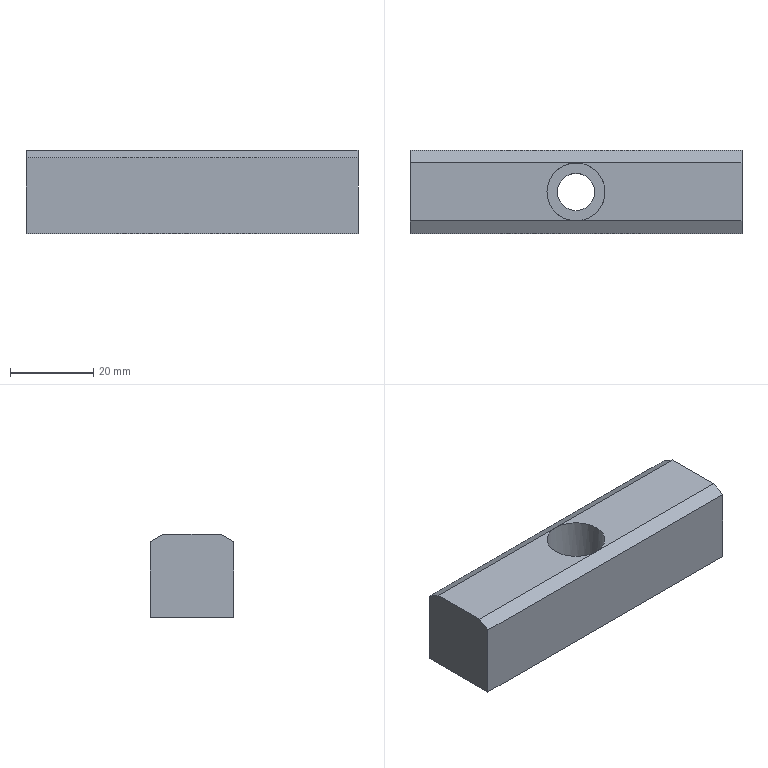Part | NX | features solid 2 | 1 solid | 12 faces | box 80 x 20 x 20 mm | volume 29409 mm3 | plane 10 | cylinder 2 | commonest cylinder face diameters 9 x1 14 x1
STEP:
#1=CARTESIAN_POINT('',(40.,347.,-95.));
#2=VERTEX_POINT('',#1);
#3=CARTESIAN_POINT('',(40.,333.,-95.));
#4=VERTEX_POINT('',#3);
#5=CARTESIAN_POINT('',(40.,350.,-95.));
#6=DIRECTION('',(0.,1.,0.));
#7=VECTOR('',#6,1000.);
#8=LINE('',#5,#7);
#9=EDGE_CURVE('',#2,#4,#8,.F.);
#10=ORIENTED_EDGE('',*,*,#9,.F.);
#11=CARTESIAN_POINT('',(0.,347.,-95.));
#12=VERTEX_POINT('',#11);
#13=CARTESIAN_POINT('',(40.,347.,-95.));
#14=DIRECTION('',(-1.,0.,0.));
#15=VECTOR('',#14,1000.);
#16=LINE('',#13,#15);
#17=EDGE_CURVE('',#2,#12,#16,.T.);
#18=ORIENTED_EDGE('',*,*,#17,.T.);
#19=CARTESIAN_POINT('',(0.,333.,-95.));
#20=VERTEX_POINT('',#19);
#21=CARTESIAN_POINT('',(0.,340.,-95.));
#22=DIRECTION('',(0.,0.,-1.));
#23=DIRECTION('',(-1.,0.,0.));
#24=AXIS2_PLACEMENT_3D('',#21,#22,#23);
#25=CIRCLE('',#24,7.);
#26=EDGE_CURVE('',#12,#20,#25,.T.);
#27=ORIENTED_EDGE('',*,*,#26,.T.);
#28=CARTESIAN_POINT('',(40.,333.,-95.));
#29=DIRECTION('',(1.,0.,0.));
#30=VECTOR('',#29,1000.);
#31=LINE('',#28,#30);
#32=EDGE_CURVE('',#20,#4,#31,.T.);
#33=ORIENTED_EDGE('',*,*,#32,.T.);
#34=EDGE_LOOP('',(#10,#18,#27,#33));
#35=FACE_BOUND('',#34,.T.);
#36=CARTESIAN_POINT('',(40.,350.,-95.));
#37=DIRECTION('',(0.,0.,1.));
#38=DIRECTION('',(1.,0.,0.));
#39=AXIS2_PLACEMENT_3D('',#36,#37,#38);
#40=PLANE('',#39);
#41=ADVANCED_FACE('',(#35),#40,.T.);
#42=CARTESIAN_POINT('',(-40.,350.,-115.));
#43=VERTEX_POINT('',#42);
#44=CARTESIAN_POINT('',(-40.,350.,-96.732));
#45=VERTEX_POINT('',#44);
#46=CARTESIAN_POINT('',(-40.,350.,-115.));
#47=DIRECTION('',(0.,0.,1.));
#48=VECTOR('',#47,1000.);
#49=LINE('',#46,#48);
#50=EDGE_CURVE('',#43,#45,#49,.T.);
#51=ORIENTED_EDGE('',*,*,#50,.T.);
#52=CARTESIAN_POINT('',(40.,350.,-96.732));
#53=VERTEX_POINT('',#52);
#54=CARTESIAN_POINT('',(40.,350.,-96.732));
#55=DIRECTION('',(1.,0.,0.));
#56=VECTOR('',#55,1000.);
#57=LINE('',#54,#56);
#58=EDGE_CURVE('',#45,#53,#57,.T.);
#59=ORIENTED_EDGE('',*,*,#58,.T.);
#60=CARTESIAN_POINT('',(40.,350.,-115.));
#61=VERTEX_POINT('',#60);
#62=CARTESIAN_POINT('',(40.,350.,-115.));
#63=DIRECTION('',(0.,0.,1.));
#64=VECTOR('',#63,1000.);
#65=LINE('',#62,#64);
#66=EDGE_CURVE('',#61,#53,#65,.T.);
#67=ORIENTED_EDGE('',*,*,#66,.F.);
#68=CARTESIAN_POINT('',(40.,350.,-115.));
#69=DIRECTION('',(-1.,0.,0.));
#70=VECTOR('',#69,1000.);
#71=LINE('',#68,#70);
#72=EDGE_CURVE('',#61,#43,#71,.T.);
#73=ORIENTED_EDGE('',*,*,#72,.T.);
#74=EDGE_LOOP('',(#51,#59,#67,#73));
#75=FACE_BOUND('',#74,.T.);
#76=CARTESIAN_POINT('',(40.,350.,-115.));
#77=DIRECTION('',(0.,1.,0.));
#78=DIRECTION('',(-1.,0.,0.));
#79=AXIS2_PLACEMENT_3D('',#76,#77,#78);
#80=PLANE('',#79);
#81=ADVANCED_FACE('',(#75),#80,.T.);
#82=CARTESIAN_POINT('',(-40.,347.,-95.));
#83=VERTEX_POINT('',#82);
#84=CARTESIAN_POINT('',(-40.,333.,-95.));
#85=VERTEX_POINT('',#84);
#86=CARTESIAN_POINT('',(-40.,350.,-95.));
#87=DIRECTION('',(0.,1.,0.));
#88=VECTOR('',#87,1000.);
#89=LINE('',#86,#88);
#90=EDGE_CURVE('',#83,#85,#89,.F.);
#91=ORIENTED_EDGE('',*,*,#90,.F.);
#92=CARTESIAN_POINT('',(-40.,357.91,-101.299));
#93=DIRECTION('',(0.,-0.866,0.5));
#94=VECTOR('',#93,1000.);
#95=LINE('',#92,#94);
#96=EDGE_CURVE('',#83,#45,#95,.F.);
#97=ORIENTED_EDGE('',*,*,#96,.T.);
#98=ORIENTED_EDGE('',*,*,#50,.F.);
#99=CARTESIAN_POINT('',(-40.,330.,-115.));
#100=VERTEX_POINT('',#99);
#101=CARTESIAN_POINT('',(-40.,350.,-115.));
#102=DIRECTION('',(0.,-1.,0.));
#103=VECTOR('',#102,1000.);
#104=LINE('',#101,#103);
#105=EDGE_CURVE('',#43,#100,#104,.T.);
#106=ORIENTED_EDGE('',*,*,#105,.T.);
#107=CARTESIAN_POINT('',(-40.,330.,-96.732));
#108=VERTEX_POINT('',#107);
#109=CARTESIAN_POINT('',(-40.,330.,-115.));
#110=DIRECTION('',(0.,0.,1.));
#111=VECTOR('',#110,1000.);
#112=LINE('',#109,#111);
#113=EDGE_CURVE('',#100,#108,#112,.T.);
#114=ORIENTED_EDGE('',*,*,#113,.T.);
#115=CARTESIAN_POINT('',(-40.,337.09,-92.639));
#116=DIRECTION('',(0.,0.866,0.5));
#117=VECTOR('',#116,1000.);
#118=LINE('',#115,#117);
#119=EDGE_CURVE('',#108,#85,#118,.T.);
#120=ORIENTED_EDGE('',*,*,#119,.T.);
#121=EDGE_LOOP('',(#91,#97,#98,#106,#114,#120));
#122=FACE_BOUND('',#121,.T.);
#123=CARTESIAN_POINT('',(-40.,350.,-115.));
#124=DIRECTION('',(-1.,0.,0.));
#125=DIRECTION('',(0.,-1.,0.));
#126=AXIS2_PLACEMENT_3D('',#123,#124,#125);
#127=PLANE('',#126);
#128=ADVANCED_FACE('',(#122),#127,.T.);
#129=CARTESIAN_POINT('',(40.,330.,-115.));
#130=VERTEX_POINT('',#129);
#131=CARTESIAN_POINT('',(40.,330.,-96.732));
#132=VERTEX_POINT('',#131);
#133=CARTESIAN_POINT('',(40.,330.,-115.));
#134=DIRECTION('',(0.,0.,1.));
#135=VECTOR('',#134,1000.);
#136=LINE('',#133,#135);
#137=EDGE_CURVE('',#130,#132,#136,.T.);
#138=ORIENTED_EDGE('',*,*,#137,.T.);
#139=CARTESIAN_POINT('',(40.,330.,-96.732));
#140=DIRECTION('',(1.,0.,0.));
#141=VECTOR('',#140,1000.);
#142=LINE('',#139,#141);
#143=EDGE_CURVE('',#132,#108,#142,.F.);
#144=ORIENTED_EDGE('',*,*,#143,.T.);
#145=ORIENTED_EDGE('',*,*,#113,.F.);
#146=CARTESIAN_POINT('',(40.,330.,-115.));
#147=DIRECTION('',(-1.,0.,0.));
#148=VECTOR('',#147,1000.);
#149=LINE('',#146,#148);
#150=EDGE_CURVE('',#130,#100,#149,.T.);
#151=ORIENTED_EDGE('',*,*,#150,.F.);
#152=EDGE_LOOP('',(#138,#144,#145,#151));
#153=FACE_BOUND('',#152,.T.);
#154=CARTESIAN_POINT('',(40.,330.,-115.));
#155=DIRECTION('',(0.,1.,0.));
#156=DIRECTION('',(-1.,0.,0.));
#157=AXIS2_PLACEMENT_3D('',#154,#155,#156);
#158=PLANE('',#157);
#159=ADVANCED_FACE('',(#153),#158,.F.);
#160=CARTESIAN_POINT('',(0.,340.,-95.));
#161=DIRECTION('',(0.,0.,-1.));
#162=DIRECTION('',(-1.,0.,0.));
#163=AXIS2_PLACEMENT_3D('',#160,#161,#162);
#164=CIRCLE('',#163,7.);
#165=EDGE_CURVE('',#20,#12,#164,.T.);
#166=ORIENTED_EDGE('',*,*,#165,.T.);
#167=CARTESIAN_POINT('',(40.,347.,-95.));
#168=DIRECTION('',(-1.,0.,0.));
#169=VECTOR('',#168,1000.);
#170=LINE('',#167,#169);
#171=EDGE_CURVE('',#12,#83,#170,.T.);
#172=ORIENTED_EDGE('',*,*,#171,.T.);
#173=ORIENTED_EDGE('',*,*,#90,.T.);
#174=CARTESIAN_POINT('',(40.,333.,-95.));
#175=DIRECTION('',(1.,0.,0.));
#176=VECTOR('',#175,1000.);
#177=LINE('',#174,#176);
#178=EDGE_CURVE('',#85,#20,#177,.T.);
#179=ORIENTED_EDGE('',*,*,#178,.T.);
#180=EDGE_LOOP('',(#166,#172,#173,#179));
#181=FACE_BOUND('',#180,.T.);
#182=CARTESIAN_POINT('',(40.,350.,-95.));
#183=DIRECTION('',(0.,0.,1.));
#184=DIRECTION('',(1.,0.,0.));
#185=AXIS2_PLACEMENT_3D('',#182,#183,#184);
#186=PLANE('',#185);
#187=ADVANCED_FACE('',(#181),#186,.T.);
#188=ORIENTED_EDGE('',*,*,#66,.T.);
#189=CARTESIAN_POINT('',(40.,357.91,-101.299));
#190=DIRECTION('',(0.,-0.866,0.5));
#191=VECTOR('',#190,1000.);
#192=LINE('',#189,#191);
#193=EDGE_CURVE('',#53,#2,#192,.T.);
#194=ORIENTED_EDGE('',*,*,#193,.T.);
#195=ORIENTED_EDGE('',*,*,#9,.T.);
#196=CARTESIAN_POINT('',(40.,337.09,-92.639));
#197=DIRECTION('',(0.,0.866,0.5));
#198=VECTOR('',#197,1000.);
#199=LINE('',#196,#198);
#200=EDGE_CURVE('',#4,#132,#199,.F.);
#201=ORIENTED_EDGE('',*,*,#200,.T.);
#202=ORIENTED_EDGE('',*,*,#137,.F.);
#203=CARTESIAN_POINT('',(40.,350.,-115.));
#204=DIRECTION('',(0.,-1.,0.));
#205=VECTOR('',#204,1000.);
#206=LINE('',#203,#205);
#207=EDGE_CURVE('',#61,#130,#206,.T.);
#208=ORIENTED_EDGE('',*,*,#207,.F.);
#209=EDGE_LOOP('',(#188,#194,#195,#201,#202,#208));
#210=FACE_BOUND('',#209,.T.);
#211=CARTESIAN_POINT('',(40.,350.,-115.));
#212=DIRECTION('',(-1.,0.,0.));
#213=DIRECTION('',(0.,-1.,0.));
#214=AXIS2_PLACEMENT_3D('',#211,#212,#213);
#215=PLANE('',#214);
#216=ADVANCED_FACE('',(#210),#215,.F.);
#217=CARTESIAN_POINT('',(4.5,340.,-115.));
#218=VERTEX_POINT('',#217);
#219=CARTESIAN_POINT('',(0.,340.,-115.));
#220=DIRECTION('',(0.,0.,1.));
#221=DIRECTION('',(1.,0.,0.));
#222=AXIS2_PLACEMENT_3D('',#219,#220,#221);
#223=CIRCLE('',#222,4.5);
#224=EDGE_CURVE('',#218,#218,#223,.T.);
#225=ORIENTED_EDGE('',*,*,#224,.T.);
#226=EDGE_LOOP('',(#225));
#227=FACE_BOUND('',#226,.T.);
#228=ORIENTED_EDGE('',*,*,#150,.T.);
#229=ORIENTED_EDGE('',*,*,#105,.F.);
#230=ORIENTED_EDGE('',*,*,#72,.F.);
#231=ORIENTED_EDGE('',*,*,#207,.T.);
#232=EDGE_LOOP('',(#228,#229,#230,#231));
#233=FACE_BOUND('',#232,.T.);
#234=CARTESIAN_POINT('',(40.,350.,-115.));
#235=DIRECTION('',(0.,0.,1.));
#236=DIRECTION('',(1.,0.,0.));
#237=AXIS2_PLACEMENT_3D('',#234,#235,#236);
#238=PLANE('',#237);
#239=ADVANCED_FACE('',(#227,#233),#238,.F.);
#240=CARTESIAN_POINT('',(-4.5,340.,-105.));
#241=VERTEX_POINT('',#240);
#242=CARTESIAN_POINT('',(0.,340.,-105.));
#243=DIRECTION('',(0.,0.,-1.));
#244=DIRECTION('',(-1.,0.,0.));
#245=AXIS2_PLACEMENT_3D('',#242,#243,#244);
#246=CIRCLE('',#245,4.5);
#247=EDGE_CURVE('',#241,#241,#246,.T.);
#248=ORIENTED_EDGE('',*,*,#247,.F.);
#249=EDGE_LOOP('',(#248));
#250=FACE_BOUND('',#249,.T.);
#251=ORIENTED_EDGE('',*,*,#224,.F.);
#252=EDGE_LOOP('',(#251));
#253=FACE_BOUND('',#252,.T.);
#254=CARTESIAN_POINT('',(0.,340.,-145.));
#255=DIRECTION('',(0.,0.,-1.));
#256=DIRECTION('',(-1.,0.,0.));
#257=AXIS2_PLACEMENT_3D('',#254,#255,#256);
#258=CYLINDRICAL_SURFACE('',#257,4.5);
#259=ADVANCED_FACE('',(#250,#253),#258,.F.);
#260=ORIENTED_EDGE('',*,*,#247,.T.);
#261=EDGE_LOOP('',(#260));
#262=FACE_BOUND('',#261,.T.);
#263=CARTESIAN_POINT('',(-7.,340.,-105.));
#264=VERTEX_POINT('',#263);
#265=CARTESIAN_POINT('',(0.,340.,-105.));
#266=DIRECTION('',(0.,0.,-1.));
#267=DIRECTION('',(-1.,0.,0.));
#268=AXIS2_PLACEMENT_3D('',#265,#266,#267);
#269=CIRCLE('',#268,7.);
#270=EDGE_CURVE('',#264,#264,#269,.T.);
#271=ORIENTED_EDGE('',*,*,#270,.F.);
#272=EDGE_LOOP('',(#271));
#273=FACE_BOUND('',#272,.T.);
#274=CARTESIAN_POINT('',(0.,340.,-105.));
#275=DIRECTION('',(0.,0.,-1.));
#276=DIRECTION('',(-1.,0.,0.));
#277=AXIS2_PLACEMENT_3D('',#274,#275,#276);
#278=PLANE('',#277);
#279=ADVANCED_FACE('',(#262,#273),#278,.F.);
#280=ORIENTED_EDGE('',*,*,#270,.T.);
#281=EDGE_LOOP('',(#280));
#282=FACE_BOUND('',#281,.T.);
#283=ORIENTED_EDGE('',*,*,#165,.F.);
#284=ORIENTED_EDGE('',*,*,#26,.F.);
#285=EDGE_LOOP('',(#283,#284));
#286=FACE_BOUND('',#285,.T.);
#287=CARTESIAN_POINT('',(0.,340.,-95.));
#288=DIRECTION('',(0.,0.,-1.));
#289=DIRECTION('',(-1.,0.,0.));
#290=AXIS2_PLACEMENT_3D('',#287,#288,#289);
#291=CYLINDRICAL_SURFACE('',#290,7.);
#292=ADVANCED_FACE('',(#282,#286),#291,.F.);
#293=ORIENTED_EDGE('',*,*,#32,.F.);
#294=ORIENTED_EDGE('',*,*,#178,.F.);
#295=ORIENTED_EDGE('',*,*,#119,.F.);
#296=ORIENTED_EDGE('',*,*,#143,.F.);
#297=ORIENTED_EDGE('',*,*,#200,.F.);
#298=EDGE_LOOP('',(#293,#294,#295,#296,#297));
#299=FACE_BOUND('',#298,.T.);
#300=CARTESIAN_POINT('',(40.,330.,-96.732));
#301=DIRECTION('',(0.,-0.5,0.866));
#302=DIRECTION('',(0.,-0.866,-0.5));
#303=AXIS2_PLACEMENT_3D('',#300,#301,#302);
#304=PLANE('',#303);
#305=ADVANCED_FACE('',(#299),#304,.T.);
#306=ORIENTED_EDGE('',*,*,#193,.F.);
#307=ORIENTED_EDGE('',*,*,#58,.F.);
#308=ORIENTED_EDGE('',*,*,#96,.F.);
#309=ORIENTED_EDGE('',*,*,#171,.F.);
#310=ORIENTED_EDGE('',*,*,#17,.F.);
#311=EDGE_LOOP('',(#306,#307,#308,#309,#310));
#312=FACE_BOUND('',#311,.T.);
#313=CARTESIAN_POINT('',(40.,347.,-95.));
#314=DIRECTION('',(0.,-0.5,-0.866));
#315=DIRECTION('',(0.,0.866,-0.5));
#316=AXIS2_PLACEMENT_3D('',#313,#314,#315);
#317=PLANE('',#316);
#318=ADVANCED_FACE('',(#312),#317,.F.);
#319=CLOSED_SHELL('',(#41,#81,#128,#159,#187,#216,#239,#259,#279,#292,#305,#318));
#320=MANIFOLD_SOLID_BREP('',#319);
#321=(LENGTH_UNIT()NAMED_UNIT(*)SI_UNIT(.MILLI.,.METRE.));
#322=UNCERTAINTY_MEASURE_WITH_UNIT(LENGTH_MEASURE(0.00001),#321,'','');
#323=(NAMED_UNIT(*)PLANE_ANGLE_UNIT()SI_UNIT($,.RADIAN.));
#324=(NAMED_UNIT(*)SI_UNIT($,.STERADIAN.)SOLID_ANGLE_UNIT());
#325=(GEOMETRIC_REPRESENTATION_CONTEXT(3)GLOBAL_UNCERTAINTY_ASSIGNED_CONTEXT((#322))GLOBAL_UNIT_ASSIGNED_CONTEXT((#321,#323,#324))REPRESENTATION_CONTEXT('',''));
#326=ADVANCED_BREP_SHAPE_REPRESENTATION('',(#320),#325);